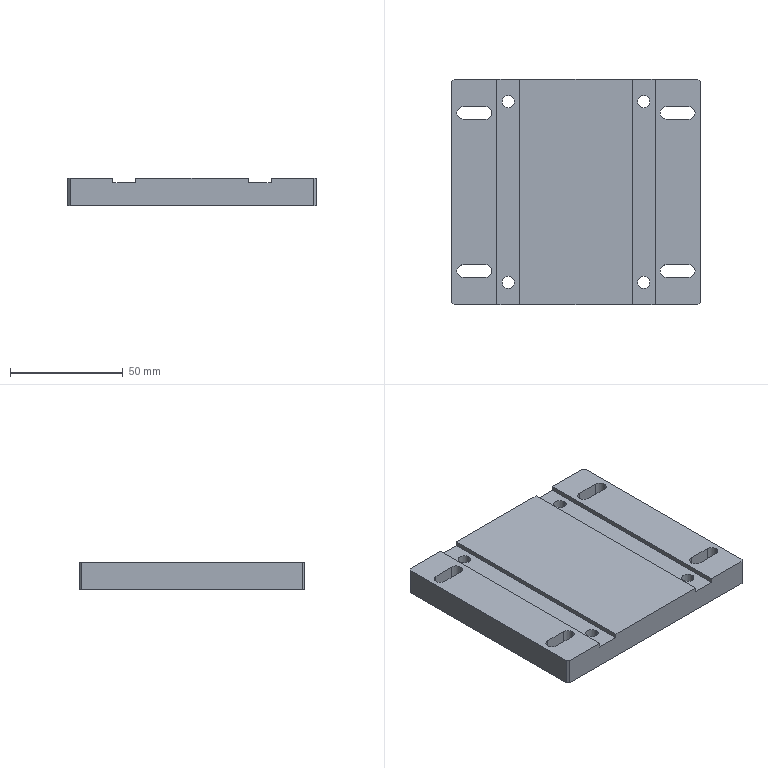Part | STEP file | PN_0035 vibratory base plate | 1 solid | 58 faces | box 110 x 100 x 12 mm | volume 122022 mm3 | plane 30 | cylinder 28 | commonest cylinder face diameters 5.5 x20 10 x8